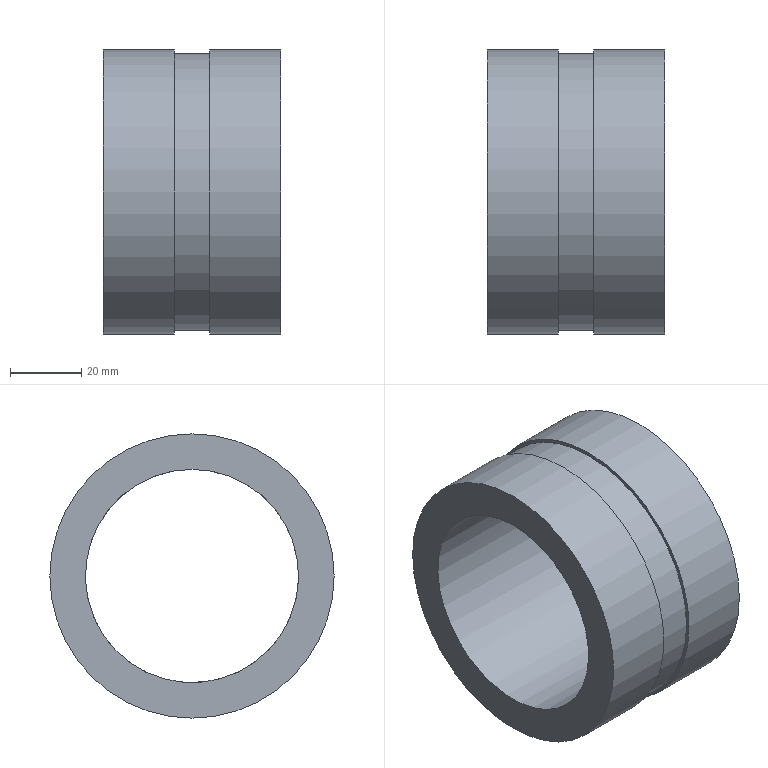Part | STEP file | solid 228 | 1 solid | 8 faces | box 50 x 80 x 80 mm | volume 107474 mm3 | cylinder 4 | plane 4 | commonest cylinder face diameters 80 x2 60 x1 78 x1